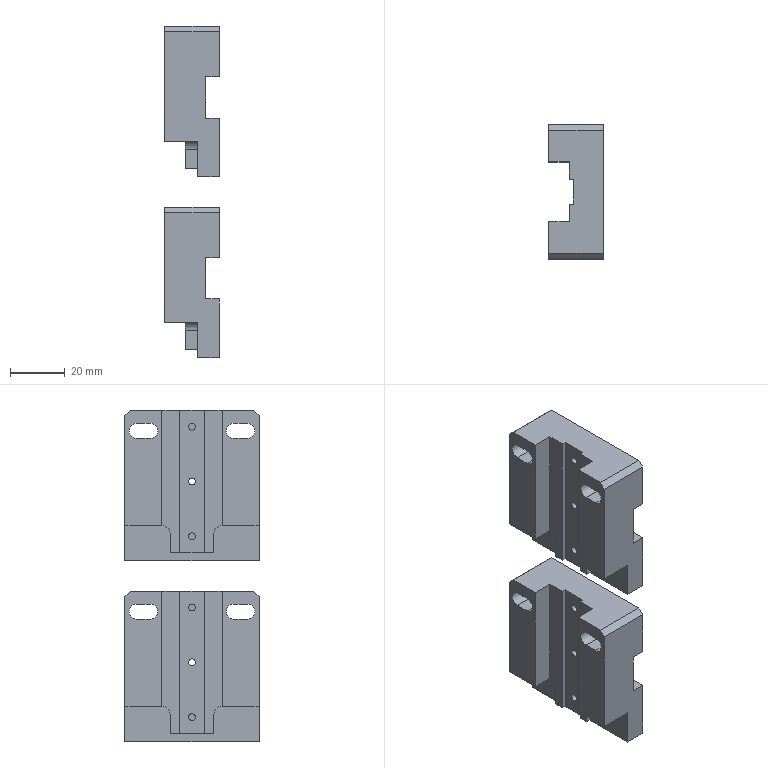Part | 2 solids | 90 faces | box 19.9 x 49 x 121 mm | volume 62645 mm3 | plane 68 | cylinder 22 | commonest cylinder face diameters 5.5 x8 2.5 x6 6 x4 9 x4